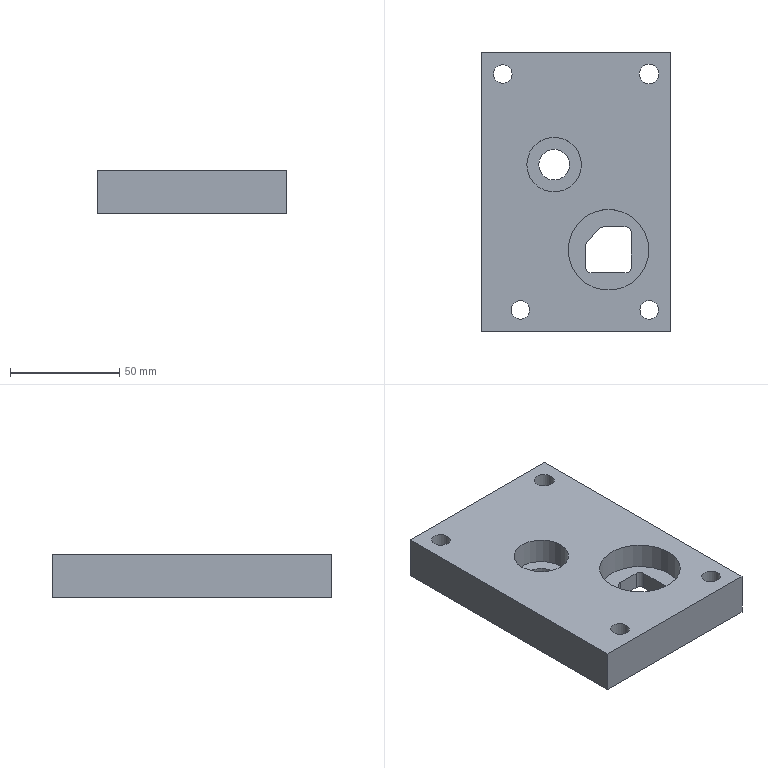Part | NX | features solid 2 | 1 solid | 33 faces | box 87 x 128 x 20 mm | volume 190901 mm3 | plane 17 | cylinder 16 | commonest cylinder face diameters 5 x5 14 x4 8.5 x3 9 x1 14.1 x1 25 x1
STEP:
#1=CARTESIAN_POINT('',(137.75,-206.5,20.));
#2=VERTEX_POINT('',#1);
#3=CARTESIAN_POINT('',(133.5,-206.5,20.));
#4=DIRECTION('',(0.,0.,1.));
#5=DIRECTION('',(1.,0.,0.));
#6=AXIS2_PLACEMENT_3D('',#3,#4,#5);
#7=CIRCLE('',#6,4.25);
#8=EDGE_CURVE('',#2,#2,#7,.F.);
#9=ORIENTED_EDGE('',*,*,#8,.T.);
#10=EDGE_LOOP('',(#9));
#11=FACE_BOUND('',#10,.T.);
#12=CARTESIAN_POINT('',(121.25,-98.5,20.));
#13=VERTEX_POINT('',#12);
#14=CARTESIAN_POINT('',(125.5,-98.5,20.));
#15=DIRECTION('',(0.,0.,1.));
#16=DIRECTION('',(-1.,0.,0.));
#17=AXIS2_PLACEMENT_3D('',#14,#15,#16);
#18=CIRCLE('',#17,4.25);
#19=EDGE_CURVE('',#13,#13,#18,.T.);
#20=ORIENTED_EDGE('',*,*,#19,.F.);
#21=EDGE_LOOP('',(#20));
#22=FACE_BOUND('',#21,.T.);
#23=CARTESIAN_POINT('',(196.75,-206.5,20.));
#24=VERTEX_POINT('',#23);
#25=CARTESIAN_POINT('',(192.5,-206.5,20.));
#26=DIRECTION('',(0.,0.,1.));
#27=DIRECTION('',(1.,0.,0.));
#28=AXIS2_PLACEMENT_3D('',#25,#26,#27);
#29=CIRCLE('',#28,4.25);
#30=EDGE_CURVE('',#24,#24,#29,.T.);
#31=ORIENTED_EDGE('',*,*,#30,.F.);
#32=EDGE_LOOP('',(#31));
#33=FACE_BOUND('',#32,.T.);
#34=CARTESIAN_POINT('',(197.,-98.5,20.));
#35=VERTEX_POINT('',#34);
#36=CARTESIAN_POINT('',(192.5,-98.5,20.));
#37=DIRECTION('',(0.,0.,-1.));
#38=DIRECTION('',(1.,0.,0.));
#39=AXIS2_PLACEMENT_3D('',#36,#37,#38);
#40=CIRCLE('',#39,4.5);
#41=EDGE_CURVE('',#35,#35,#40,.F.);
#42=ORIENTED_EDGE('',*,*,#41,.F.);
#43=EDGE_LOOP('',(#42));
#44=FACE_BOUND('',#43,.T.);
#45=CARTESIAN_POINT('',(202.5,-216.5,20.));
#46=VERTEX_POINT('',#45);
#47=CARTESIAN_POINT('',(115.5,-216.5,20.));
#48=VERTEX_POINT('',#47);
#49=CARTESIAN_POINT('',(149.,-216.5,20.));
#50=DIRECTION('',(1.,0.,0.));
#51=VECTOR('',#50,1000.);
#52=LINE('',#49,#51);
#53=EDGE_CURVE('',#46,#48,#52,.F.);
#54=ORIENTED_EDGE('',*,*,#53,.F.);
#55=CARTESIAN_POINT('',(202.5,-88.5,20.));
#56=VERTEX_POINT('',#55);
#57=CARTESIAN_POINT('',(202.5,-140.,20.));
#58=DIRECTION('',(0.,-1.,0.));
#59=VECTOR('',#58,1000.);
#60=LINE('',#57,#59);
#61=EDGE_CURVE('',#56,#46,#60,.T.);
#62=ORIENTED_EDGE('',*,*,#61,.F.);
#63=CARTESIAN_POINT('',(115.5,-88.5,20.));
#64=VERTEX_POINT('',#63);
#65=CARTESIAN_POINT('',(149.,-88.5,20.));
#66=DIRECTION('',(1.,0.,0.));
#67=VECTOR('',#66,1000.);
#68=LINE('',#65,#67);
#69=EDGE_CURVE('',#64,#56,#68,.T.);
#70=ORIENTED_EDGE('',*,*,#69,.F.);
#71=CARTESIAN_POINT('',(115.5,-140.,20.));
#72=DIRECTION('',(0.,1.,0.));
#73=VECTOR('',#72,1000.);
#74=LINE('',#71,#73);
#75=EDGE_CURVE('',#48,#64,#74,.T.);
#76=ORIENTED_EDGE('',*,*,#75,.F.);
#77=EDGE_LOOP('',(#54,#62,#70,#76));
#78=FACE_BOUND('',#77,.T.);
#79=CARTESIAN_POINT('',(161.5,-140.,20.));
#80=VERTEX_POINT('',#79);
#81=CARTESIAN_POINT('',(149.,-140.,20.));
#82=DIRECTION('',(0.,0.,1.));
#83=DIRECTION('',(1.,0.,0.));
#84=AXIS2_PLACEMENT_3D('',#81,#82,#83);
#85=CIRCLE('',#84,12.5);
#86=EDGE_CURVE('',#80,#80,#85,.T.);
#87=ORIENTED_EDGE('',*,*,#86,.F.);
#88=EDGE_LOOP('',(#87));
#89=FACE_BOUND('',#88,.T.);
#90=CARTESIAN_POINT('',(192.401,-179.,20.));
#91=VERTEX_POINT('',#90);
#92=CARTESIAN_POINT('',(173.901,-179.,20.));
#93=DIRECTION('',(0.,0.,1.));
#94=DIRECTION('',(1.,0.,0.));
#95=AXIS2_PLACEMENT_3D('',#92,#93,#94);
#96=CIRCLE('',#95,18.5);
#97=EDGE_CURVE('',#91,#91,#96,.T.);
#98=ORIENTED_EDGE('',*,*,#97,.F.);
#99=EDGE_LOOP('',(#98));
#100=FACE_BOUND('',#99,.T.);
#101=CARTESIAN_POINT('',(251.29,-25.984,20.));
#102=DIRECTION('',(0.,0.,1.));
#103=DIRECTION('',(1.,0.,0.));
#104=AXIS2_PLACEMENT_3D('',#101,#102,#103);
#105=PLANE('',#104);
#106=ADVANCED_FACE('',(#11,#22,#33,#44,#78,#89,#100),#105,.T.);
#107=CARTESIAN_POINT('',(185.5,-98.5,0.00000121));
#108=VERTEX_POINT('',#107);
#109=CARTESIAN_POINT('',(192.5,-98.5,0.00000121));
#110=DIRECTION('',(0.,0.,1.));
#111=DIRECTION('',(-1.,0.,0.));
#112=AXIS2_PLACEMENT_3D('',#109,#110,#111);
#113=CIRCLE('',#112,7.);
#114=EDGE_CURVE('',#108,#108,#113,.F.);
#115=ORIENTED_EDGE('',*,*,#114,.F.);
#116=EDGE_LOOP('',(#115));
#117=FACE_BOUND('',#116,.T.);
#118=CARTESIAN_POINT('',(141.95,-140.,0.00000121));
#119=VERTEX_POINT('',#118);
#120=CARTESIAN_POINT('',(149.,-140.,0.00000121));
#121=DIRECTION('',(0.,0.,1.));
#122=DIRECTION('',(-1.,0.,0.));
#123=AXIS2_PLACEMENT_3D('',#120,#121,#122);
#124=CIRCLE('',#123,7.05);
#125=EDGE_CURVE('',#119,#119,#124,.F.);
#126=ORIENTED_EDGE('',*,*,#125,.F.);
#127=EDGE_LOOP('',(#126));
#128=FACE_BOUND('',#127,.T.);
#129=CARTESIAN_POINT('',(185.5,-206.5,0.00000121));
#130=VERTEX_POINT('',#129);
#131=CARTESIAN_POINT('',(192.5,-206.5,0.00000121));
#132=DIRECTION('',(0.,0.,-1.));
#133=DIRECTION('',(-1.,0.,0.));
#134=AXIS2_PLACEMENT_3D('',#131,#132,#133);
#135=CIRCLE('',#134,7.);
#136=EDGE_CURVE('',#130,#130,#135,.T.);
#137=ORIENTED_EDGE('',*,*,#136,.F.);
#138=EDGE_LOOP('',(#137));
#139=FACE_BOUND('',#138,.T.);
#140=CARTESIAN_POINT('',(202.5,-88.5,0.00000121));
#141=VERTEX_POINT('',#140);
#142=CARTESIAN_POINT('',(202.5,-216.5,0.00000121));
#143=VERTEX_POINT('',#142);
#144=CARTESIAN_POINT('',(202.5,-140.,0.00000121));
#145=DIRECTION('',(0.,1.,0.));
#146=VECTOR('',#145,1000.);
#147=LINE('',#144,#146);
#148=EDGE_CURVE('',#141,#143,#147,.F.);
#149=ORIENTED_EDGE('',*,*,#148,.T.);
#150=CARTESIAN_POINT('',(115.5,-216.5,0.00000121));
#151=VERTEX_POINT('',#150);
#152=CARTESIAN_POINT('',(149.,-216.5,0.00000121));
#153=DIRECTION('',(-1.,0.,0.));
#154=VECTOR('',#153,1000.);
#155=LINE('',#152,#154);
#156=EDGE_CURVE('',#143,#151,#155,.T.);
#157=ORIENTED_EDGE('',*,*,#156,.T.);
#158=CARTESIAN_POINT('',(115.5,-88.5,0.00000121));
#159=VERTEX_POINT('',#158);
#160=CARTESIAN_POINT('',(115.5,-140.,0.00000121));
#161=DIRECTION('',(0.,-1.,0.));
#162=VECTOR('',#161,1000.);
#163=LINE('',#160,#162);
#164=EDGE_CURVE('',#151,#159,#163,.F.);
#165=ORIENTED_EDGE('',*,*,#164,.T.);
#166=CARTESIAN_POINT('',(149.,-88.5,0.00000121));
#167=DIRECTION('',(-1.,0.,0.));
#168=VECTOR('',#167,1000.);
#169=LINE('',#166,#168);
#170=EDGE_CURVE('',#159,#141,#169,.F.);
#171=ORIENTED_EDGE('',*,*,#170,.T.);
#172=EDGE_LOOP('',(#149,#157,#165,#171));
#173=FACE_BOUND('',#172,.T.);
#174=CARTESIAN_POINT('',(132.5,-98.5,0.00000121));
#175=VERTEX_POINT('',#174);
#176=CARTESIAN_POINT('',(125.5,-98.5,0.00000121));
#177=DIRECTION('',(0.,0.,-1.));
#178=DIRECTION('',(1.,0.,0.));
#179=AXIS2_PLACEMENT_3D('',#176,#177,#178);
#180=CIRCLE('',#179,7.);
#181=EDGE_CURVE('',#175,#175,#180,.T.);
#182=ORIENTED_EDGE('',*,*,#181,.F.);
#183=EDGE_LOOP('',(#182));
#184=FACE_BOUND('',#183,.T.);
#185=CARTESIAN_POINT('',(126.5,-206.5,0.00000121));
#186=VERTEX_POINT('',#185);
#187=CARTESIAN_POINT('',(133.5,-206.5,0.00000121));
#188=DIRECTION('',(0.,0.,-1.));
#189=DIRECTION('',(-1.,0.,0.));
#190=AXIS2_PLACEMENT_3D('',#187,#188,#189);
#191=CIRCLE('',#190,7.);
#192=EDGE_CURVE('',#186,#186,#191,.T.);
#193=ORIENTED_EDGE('',*,*,#192,.F.);
#194=EDGE_LOOP('',(#193));
#195=FACE_BOUND('',#194,.T.);
#196=CARTESIAN_POINT('',(184.401,-171.,0.00000121));
#197=VERTEX_POINT('',#196);
#198=CARTESIAN_POINT('',(181.901,-168.5,0.00000121));
#199=VERTEX_POINT('',#198);
#200=CARTESIAN_POINT('',(181.901,-171.,0.00000121));
#201=DIRECTION('',(0.,0.,-1.));
#202=DIRECTION('',(-1.,0.,0.));
#203=AXIS2_PLACEMENT_3D('',#200,#201,#202);
#204=CIRCLE('',#203,2.5);
#205=EDGE_CURVE('',#197,#199,#204,.F.);
#206=ORIENTED_EDGE('',*,*,#205,.T.);
#207=CARTESIAN_POINT('',(171.729,-168.5,0.00000121));
#208=VERTEX_POINT('',#207);
#209=CARTESIAN_POINT('',(149.,-168.5,0.00000121));
#210=DIRECTION('',(-1.,0.,0.));
#211=VECTOR('',#210,1000.);
#212=LINE('',#209,#211);
#213=EDGE_CURVE('',#199,#208,#212,.T.);
#214=ORIENTED_EDGE('',*,*,#213,.T.);
#215=CARTESIAN_POINT('',(169.961,-169.232,0.00000121));
#216=VERTEX_POINT('',#215);
#217=CARTESIAN_POINT('',(171.729,-171.,0.00000121));
#218=DIRECTION('',(0.,0.,-1.));
#219=DIRECTION('',(-1.,0.,0.));
#220=AXIS2_PLACEMENT_3D('',#217,#218,#219);
#221=CIRCLE('',#220,2.5);
#222=EDGE_CURVE('',#208,#216,#221,.F.);
#223=ORIENTED_EDGE('',*,*,#222,.T.);
#224=CARTESIAN_POINT('',(164.133,-175.061,0.00000121));
#225=VERTEX_POINT('',#224);
#226=CARTESIAN_POINT('',(174.097,-165.097,0.00000121));
#227=DIRECTION('',(-0.7071,-0.7071,0.));
#228=VECTOR('',#227,1000.);
#229=LINE('',#226,#228);
#230=EDGE_CURVE('',#216,#225,#229,.T.);
#231=ORIENTED_EDGE('',*,*,#230,.T.);
#232=CARTESIAN_POINT('',(163.401,-176.828,0.00000121));
#233=VERTEX_POINT('',#232);
#234=CARTESIAN_POINT('',(165.901,-176.828,0.00000121));
#235=DIRECTION('',(0.,0.,-1.));
#236=DIRECTION('',(-1.,0.,0.));
#237=AXIS2_PLACEMENT_3D('',#234,#235,#236);
#238=CIRCLE('',#237,2.5);
#239=EDGE_CURVE('',#225,#233,#238,.F.);
#240=ORIENTED_EDGE('',*,*,#239,.T.);
#241=CARTESIAN_POINT('',(163.401,-187.,0.00000121));
#242=VERTEX_POINT('',#241);
#243=CARTESIAN_POINT('',(163.401,-140.,0.00000121));
#244=DIRECTION('',(0.,-1.,0.));
#245=VECTOR('',#244,1000.);
#246=LINE('',#243,#245);
#247=EDGE_CURVE('',#233,#242,#246,.T.);
#248=ORIENTED_EDGE('',*,*,#247,.T.);
#249=CARTESIAN_POINT('',(165.901,-189.5,0.00000121));
#250=VERTEX_POINT('',#249);
#251=CARTESIAN_POINT('',(165.901,-187.,0.00000121));
#252=DIRECTION('',(0.,0.,-1.));
#253=DIRECTION('',(-1.,0.,0.));
#254=AXIS2_PLACEMENT_3D('',#251,#252,#253);
#255=CIRCLE('',#254,2.5);
#256=EDGE_CURVE('',#242,#250,#255,.F.);
#257=ORIENTED_EDGE('',*,*,#256,.T.);
#258=CARTESIAN_POINT('',(181.901,-189.5,0.00000121));
#259=VERTEX_POINT('',#258);
#260=CARTESIAN_POINT('',(149.,-189.5,0.00000121));
#261=DIRECTION('',(1.,0.,0.));
#262=VECTOR('',#261,1000.);
#263=LINE('',#260,#262);
#264=EDGE_CURVE('',#250,#259,#263,.T.);
#265=ORIENTED_EDGE('',*,*,#264,.T.);
#266=CARTESIAN_POINT('',(184.401,-187.,0.00000121));
#267=VERTEX_POINT('',#266);
#268=CARTESIAN_POINT('',(181.901,-187.,0.00000121));
#269=DIRECTION('',(0.,0.,-1.));
#270=DIRECTION('',(-1.,0.,0.));
#271=AXIS2_PLACEMENT_3D('',#268,#269,#270);
#272=CIRCLE('',#271,2.5);
#273=EDGE_CURVE('',#259,#267,#272,.F.);
#274=ORIENTED_EDGE('',*,*,#273,.T.);
#275=CARTESIAN_POINT('',(184.401,-140.,0.00000121));
#276=DIRECTION('',(0.,1.,0.));
#277=VECTOR('',#276,1000.);
#278=LINE('',#275,#277);
#279=EDGE_CURVE('',#267,#197,#278,.T.);
#280=ORIENTED_EDGE('',*,*,#279,.T.);
#281=EDGE_LOOP('',(#206,#214,#223,#231,#240,#248,#257,#265,#274,#280));
#282=FACE_BOUND('',#281,.T.);
#283=CARTESIAN_POINT('',(149.,-140.,0.00000121));
#284=DIRECTION('',(0.,0.,-1.));
#285=DIRECTION('',(-1.,0.,0.));
#286=AXIS2_PLACEMENT_3D('',#283,#284,#285);
#287=PLANE('',#286);
#288=ADVANCED_FACE('',(#117,#128,#139,#173,#184,#195,#282),#287,.T.);
#289=CARTESIAN_POINT('',(129.25,-206.5,10.));
#290=VERTEX_POINT('',#289);
#291=CARTESIAN_POINT('',(133.5,-206.5,10.));
#292=DIRECTION('',(0.,0.,-1.));
#293=DIRECTION('',(-1.,0.,0.));
#294=AXIS2_PLACEMENT_3D('',#291,#292,#293);
#295=CIRCLE('',#294,4.25);
#296=EDGE_CURVE('',#290,#290,#295,.F.);
#297=ORIENTED_EDGE('',*,*,#296,.T.);
#298=EDGE_LOOP('',(#297));
#299=FACE_BOUND('',#298,.T.);
#300=CARTESIAN_POINT('',(126.5,-206.5,10.));
#301=VERTEX_POINT('',#300);
#302=CARTESIAN_POINT('',(133.5,-206.5,10.));
#303=DIRECTION('',(0.,0.,-1.));
#304=DIRECTION('',(-1.,0.,0.));
#305=AXIS2_PLACEMENT_3D('',#302,#303,#304);
#306=CIRCLE('',#305,7.);
#307=EDGE_CURVE('',#301,#301,#306,.F.);
#308=ORIENTED_EDGE('',*,*,#307,.F.);
#309=EDGE_LOOP('',(#308));
#310=FACE_BOUND('',#309,.T.);
#311=CARTESIAN_POINT('',(19.595,-220.431,10.));
#312=DIRECTION('',(0.,0.,1.));
#313=DIRECTION('',(-1.,0.,0.));
#314=AXIS2_PLACEMENT_3D('',#311,#312,#313);
#315=PLANE('',#314);
#316=ADVANCED_FACE('',(#299,#310),#315,.F.);
#317=ORIENTED_EDGE('',*,*,#8,.F.);
#318=EDGE_LOOP('',(#317));
#319=FACE_BOUND('',#318,.T.);
#320=ORIENTED_EDGE('',*,*,#296,.F.);
#321=EDGE_LOOP('',(#320));
#322=FACE_BOUND('',#321,.T.);
#323=CARTESIAN_POINT('',(133.5,-206.5,35.));
#324=DIRECTION('',(0.,0.,1.));
#325=DIRECTION('',(1.,0.,0.));
#326=AXIS2_PLACEMENT_3D('',#323,#324,#325);
#327=CYLINDRICAL_SURFACE('',#326,4.25);
#328=ADVANCED_FACE('',(#319,#322),#327,.F.);
#329=ORIENTED_EDGE('',*,*,#307,.T.);
#330=EDGE_LOOP('',(#329));
#331=FACE_BOUND('',#330,.T.);
#332=ORIENTED_EDGE('',*,*,#192,.T.);
#333=EDGE_LOOP('',(#332));
#334=FACE_BOUND('',#333,.T.);
#335=CARTESIAN_POINT('',(133.5,-206.5,0.00000121));
#336=DIRECTION('',(0.,0.,1.));
#337=DIRECTION('',(1.,0.,0.));
#338=AXIS2_PLACEMENT_3D('',#335,#336,#337);
#339=CYLINDRICAL_SURFACE('',#338,7.);
#340=ADVANCED_FACE('',(#331,#334),#339,.F.);
#341=CARTESIAN_POINT('',(197.,-98.5,10.));
#342=VERTEX_POINT('',#341);
#343=CARTESIAN_POINT('',(192.5,-98.5,10.));
#344=DIRECTION('',(0.,0.,-1.));
#345=DIRECTION('',(1.,0.,0.));
#346=AXIS2_PLACEMENT_3D('',#343,#344,#345);
#347=CIRCLE('',#346,4.5);
#348=EDGE_CURVE('',#342,#342,#347,.F.);
#349=ORIENTED_EDGE('',*,*,#348,.T.);
#350=EDGE_LOOP('',(#349));
#351=FACE_BOUND('',#350,.T.);
#352=CARTESIAN_POINT('',(199.5,-98.5,10.));
#353=VERTEX_POINT('',#352);
#354=CARTESIAN_POINT('',(192.5,-98.5,10.));
#355=DIRECTION('',(0.,0.,-1.));
#356=DIRECTION('',(1.,0.,0.));
#357=AXIS2_PLACEMENT_3D('',#354,#355,#356);
#358=CIRCLE('',#357,7.);
#359=EDGE_CURVE('',#353,#353,#358,.F.);
#360=ORIENTED_EDGE('',*,*,#359,.F.);
#361=EDGE_LOOP('',(#360));
#362=FACE_BOUND('',#361,.T.);
#363=CARTESIAN_POINT('',(306.405,-84.569,10.));
#364=DIRECTION('',(0.,0.,1.));
#365=DIRECTION('',(1.,0.,0.));
#366=AXIS2_PLACEMENT_3D('',#363,#364,#365);
#367=PLANE('',#366);
#368=ADVANCED_FACE('',(#351,#362),#367,.F.);
#369=CARTESIAN_POINT('',(161.5,-140.,8.));
#370=VERTEX_POINT('',#369);
#371=CARTESIAN_POINT('',(149.,-140.,8.));
#372=DIRECTION('',(0.,0.,1.));
#373=DIRECTION('',(1.,0.,0.));
#374=AXIS2_PLACEMENT_3D('',#371,#372,#373);
#375=CIRCLE('',#374,12.5);
#376=EDGE_CURVE('',#370,#370,#375,.T.);
#377=ORIENTED_EDGE('',*,*,#376,.T.);
#378=EDGE_LOOP('',(#377));
#379=FACE_BOUND('',#378,.T.);
#380=CARTESIAN_POINT('',(156.05,-140.,8.));
#381=VERTEX_POINT('',#380);
#382=CARTESIAN_POINT('',(149.,-140.,8.));
#383=DIRECTION('',(0.,0.,1.));
#384=DIRECTION('',(1.,0.,0.));
#385=AXIS2_PLACEMENT_3D('',#382,#383,#384);
#386=CIRCLE('',#385,7.05);
#387=EDGE_CURVE('',#381,#381,#386,.F.);
#388=ORIENTED_EDGE('',*,*,#387,.T.);
#389=EDGE_LOOP('',(#388));
#390=FACE_BOUND('',#389,.T.);
#391=CARTESIAN_POINT('',(151.5,140.,8.));
#392=DIRECTION('',(0.,0.,1.));
#393=DIRECTION('',(1.,0.,0.));
#394=AXIS2_PLACEMENT_3D('',#391,#392,#393);
#395=PLANE('',#394);
#396=ADVANCED_FACE('',(#379,#390),#395,.T.);
#397=CARTESIAN_POINT('',(196.75,-206.5,10.));
#398=VERTEX_POINT('',#397);
#399=CARTESIAN_POINT('',(192.5,-206.5,10.));
#400=DIRECTION('',(0.,0.,1.));
#401=DIRECTION('',(1.,0.,0.));
#402=AXIS2_PLACEMENT_3D('',#399,#400,#401);
#403=CIRCLE('',#402,4.25);
#404=EDGE_CURVE('',#398,#398,#403,.T.);
#405=ORIENTED_EDGE('',*,*,#404,.T.);
#406=EDGE_LOOP('',(#405));
#407=FACE_BOUND('',#406,.T.);
#408=CARTESIAN_POINT('',(199.5,-206.5,10.));
#409=VERTEX_POINT('',#408);
#410=CARTESIAN_POINT('',(192.5,-206.5,10.));
#411=DIRECTION('',(0.,0.,1.));
#412=DIRECTION('',(1.,0.,0.));
#413=AXIS2_PLACEMENT_3D('',#410,#411,#412);
#414=CIRCLE('',#413,7.);
#415=EDGE_CURVE('',#409,#409,#414,.T.);
#416=ORIENTED_EDGE('',*,*,#415,.F.);
#417=EDGE_LOOP('',(#416));
#418=FACE_BOUND('',#417,.T.);
#419=CARTESIAN_POINT('',(306.405,-220.431,10.));
#420=DIRECTION('',(0.,0.,1.));
#421=DIRECTION('',(1.,0.,0.));
#422=AXIS2_PLACEMENT_3D('',#419,#420,#421);
#423=PLANE('',#422);
#424=ADVANCED_FACE('',(#407,#418),#423,.F.);
#425=CARTESIAN_POINT('',(121.25,-98.5,10.));
#426=VERTEX_POINT('',#425);
#427=CARTESIAN_POINT('',(125.5,-98.5,10.));
#428=DIRECTION('',(0.,0.,1.));
#429=DIRECTION('',(-1.,0.,0.));
#430=AXIS2_PLACEMENT_3D('',#427,#428,#429);
#431=CIRCLE('',#430,4.25);
#432=EDGE_CURVE('',#426,#426,#431,.T.);
#433=ORIENTED_EDGE('',*,*,#432,.T.);
#434=EDGE_LOOP('',(#433));
#435=FACE_BOUND('',#434,.T.);
#436=CARTESIAN_POINT('',(118.5,-98.5,10.));
#437=VERTEX_POINT('',#436);
#438=CARTESIAN_POINT('',(125.5,-98.5,10.));
#439=DIRECTION('',(0.,0.,1.));
#440=DIRECTION('',(-1.,0.,0.));
#441=AXIS2_PLACEMENT_3D('',#438,#439,#440);
#442=CIRCLE('',#441,7.);
#443=EDGE_CURVE('',#437,#437,#442,.T.);
#444=ORIENTED_EDGE('',*,*,#443,.F.);
#445=EDGE_LOOP('',(#444));
#446=FACE_BOUND('',#445,.T.);
#447=CARTESIAN_POINT('',(11.595,-84.569,10.));
#448=DIRECTION('',(0.,0.,1.));
#449=DIRECTION('',(-1.,0.,0.));
#450=AXIS2_PLACEMENT_3D('',#447,#448,#449);
#451=PLANE('',#450);
#452=ADVANCED_FACE('',(#435,#446),#451,.F.);
#453=ORIENTED_EDGE('',*,*,#376,.F.);
#454=EDGE_LOOP('',(#453));
#455=FACE_BOUND('',#454,.T.);
#456=ORIENTED_EDGE('',*,*,#86,.T.);
#457=EDGE_LOOP('',(#456));
#458=FACE_BOUND('',#457,.T.);
#459=CARTESIAN_POINT('',(149.,-140.,2.5));
#460=DIRECTION('',(0.,0.,-1.));
#461=DIRECTION('',(-1.,0.,0.));
#462=AXIS2_PLACEMENT_3D('',#459,#460,#461);
#463=CYLINDRICAL_SURFACE('',#462,12.5);
#464=ADVANCED_FACE('',(#455,#458),#463,.F.);
#465=ORIENTED_EDGE('',*,*,#359,.T.);
#466=EDGE_LOOP('',(#465));
#467=FACE_BOUND('',#466,.T.);
#468=ORIENTED_EDGE('',*,*,#114,.T.);
#469=EDGE_LOOP('',(#468));
#470=FACE_BOUND('',#469,.T.);
#471=CARTESIAN_POINT('',(192.5,-98.5,0.00000121));
#472=DIRECTION('',(0.,0.,1.));
#473=DIRECTION('',(-1.,0.,0.));
#474=AXIS2_PLACEMENT_3D('',#471,#472,#473);
#475=CYLINDRICAL_SURFACE('',#474,7.);
#476=ADVANCED_FACE('',(#467,#470),#475,.F.);
#477=ORIENTED_EDGE('',*,*,#125,.T.);
#478=EDGE_LOOP('',(#477));
#479=FACE_BOUND('',#478,.T.);
#480=ORIENTED_EDGE('',*,*,#387,.F.);
#481=EDGE_LOOP('',(#480));
#482=FACE_BOUND('',#481,.T.);
#483=CARTESIAN_POINT('',(149.,-140.,2.5));
#484=DIRECTION('',(0.,0.,-1.));
#485=DIRECTION('',(-1.,0.,0.));
#486=AXIS2_PLACEMENT_3D('',#483,#484,#485);
#487=CYLINDRICAL_SURFACE('',#486,7.05);
#488=ADVANCED_FACE('',(#479,#482),#487,.F.);
#489=ORIENTED_EDGE('',*,*,#415,.T.);
#490=EDGE_LOOP('',(#489));
#491=FACE_BOUND('',#490,.T.);
#492=ORIENTED_EDGE('',*,*,#136,.T.);
#493=EDGE_LOOP('',(#492));
#494=FACE_BOUND('',#493,.T.);
#495=CARTESIAN_POINT('',(192.5,-206.5,0.00000121));
#496=DIRECTION('',(0.,0.,1.));
#497=DIRECTION('',(-1.,0.,0.));
#498=AXIS2_PLACEMENT_3D('',#495,#496,#497);
#499=CYLINDRICAL_SURFACE('',#498,7.);
#500=ADVANCED_FACE('',(#491,#494),#499,.F.);
#501=CARTESIAN_POINT('',(202.5,-88.5,35.));
#502=DIRECTION('',(0.,0.,-1.));
#503=VECTOR('',#502,1000.);
#504=LINE('',#501,#503);
#505=EDGE_CURVE('',#56,#141,#504,.T.);
#506=ORIENTED_EDGE('',*,*,#505,.T.);
#507=ORIENTED_EDGE('',*,*,#170,.F.);
#508=CARTESIAN_POINT('',(115.5,-88.5,35.));
#509=DIRECTION('',(0.,0.,-1.));
#510=VECTOR('',#509,1000.);
#511=LINE('',#508,#510);
#512=EDGE_CURVE('',#64,#159,#511,.T.);
#513=ORIENTED_EDGE('',*,*,#512,.F.);
#514=ORIENTED_EDGE('',*,*,#69,.T.);
#515=EDGE_LOOP('',(#506,#507,#513,#514));
#516=FACE_BOUND('',#515,.T.);
#517=CARTESIAN_POINT('',(149.,-88.5,35.));
#518=DIRECTION('',(0.,-1.,0.));
#519=DIRECTION('',(1.,0.,0.));
#520=AXIS2_PLACEMENT_3D('',#517,#518,#519);
#521=PLANE('',#520);
#522=ADVANCED_FACE('',(#516),#521,.F.);
#523=ORIENTED_EDGE('',*,*,#512,.T.);
#524=ORIENTED_EDGE('',*,*,#164,.F.);
#525=CARTESIAN_POINT('',(115.5,-216.5,35.));
#526=DIRECTION('',(0.,0.,-1.));
#527=VECTOR('',#526,1000.);
#528=LINE('',#525,#527);
#529=EDGE_CURVE('',#151,#48,#528,.F.);
#530=ORIENTED_EDGE('',*,*,#529,.T.);
#531=ORIENTED_EDGE('',*,*,#75,.T.);
#532=EDGE_LOOP('',(#523,#524,#530,#531));
#533=FACE_BOUND('',#532,.T.);
#534=CARTESIAN_POINT('',(115.5,-140.,35.));
#535=DIRECTION('',(1.,0.,0.));
#536=DIRECTION('',(0.,1.,0.));
#537=AXIS2_PLACEMENT_3D('',#534,#535,#536);
#538=PLANE('',#537);
#539=ADVANCED_FACE('',(#533),#538,.F.);
#540=ORIENTED_EDGE('',*,*,#529,.F.);
#541=ORIENTED_EDGE('',*,*,#156,.F.);
#542=CARTESIAN_POINT('',(202.5,-216.5,35.));
#543=DIRECTION('',(0.,0.,-1.));
#544=VECTOR('',#543,1000.);
#545=LINE('',#542,#544);
#546=EDGE_CURVE('',#46,#143,#545,.T.);
#547=ORIENTED_EDGE('',*,*,#546,.F.);
#548=ORIENTED_EDGE('',*,*,#53,.T.);
#549=EDGE_LOOP('',(#540,#541,#547,#548));
#550=FACE_BOUND('',#549,.T.);
#551=CARTESIAN_POINT('',(149.,-216.5,35.));
#552=DIRECTION('',(0.,1.,0.));
#553=DIRECTION('',(-1.,0.,0.));
#554=AXIS2_PLACEMENT_3D('',#551,#552,#553);
#555=PLANE('',#554);
#556=ADVANCED_FACE('',(#550),#555,.F.);
#557=ORIENTED_EDGE('',*,*,#546,.T.);
#558=ORIENTED_EDGE('',*,*,#148,.F.);
#559=ORIENTED_EDGE('',*,*,#505,.F.);
#560=ORIENTED_EDGE('',*,*,#61,.T.);
#561=EDGE_LOOP('',(#557,#558,#559,#560));
#562=FACE_BOUND('',#561,.T.);
#563=CARTESIAN_POINT('',(202.5,-140.,35.));
#564=DIRECTION('',(-1.,0.,0.));
#565=DIRECTION('',(0.,-1.,0.));
#566=AXIS2_PLACEMENT_3D('',#563,#564,#565);
#567=PLANE('',#566);
#568=ADVANCED_FACE('',(#562),#567,.F.);
#569=ORIENTED_EDGE('',*,*,#443,.T.);
#570=EDGE_LOOP('',(#569));
#571=FACE_BOUND('',#570,.T.);
#572=ORIENTED_EDGE('',*,*,#181,.T.);
#573=EDGE_LOOP('',(#572));
#574=FACE_BOUND('',#573,.T.);
#575=CARTESIAN_POINT('',(125.5,-98.5,0.00000121));
#576=DIRECTION('',(0.,0.,1.));
#577=DIRECTION('',(1.,0.,0.));
#578=AXIS2_PLACEMENT_3D('',#575,#576,#577);
#579=CYLINDRICAL_SURFACE('',#578,7.);
#580=ADVANCED_FACE('',(#571,#574),#579,.F.);
#581=ORIENTED_EDGE('',*,*,#41,.T.);
#582=EDGE_LOOP('',(#581));
#583=FACE_BOUND('',#582,.T.);
#584=ORIENTED_EDGE('',*,*,#348,.F.);
#585=EDGE_LOOP('',(#584));
#586=FACE_BOUND('',#585,.T.);
#587=CARTESIAN_POINT('',(192.5,-98.5,35.));
#588=DIRECTION('',(0.,0.,1.));
#589=DIRECTION('',(-1.,0.,0.));
#590=AXIS2_PLACEMENT_3D('',#587,#588,#589);
#591=CYLINDRICAL_SURFACE('',#590,4.5);
#592=ADVANCED_FACE('',(#583,#586),#591,.F.);
#593=ORIENTED_EDGE('',*,*,#30,.T.);
#594=EDGE_LOOP('',(#593));
#595=FACE_BOUND('',#594,.T.);
#596=ORIENTED_EDGE('',*,*,#404,.F.);
#597=EDGE_LOOP('',(#596));
#598=FACE_BOUND('',#597,.T.);
#599=CARTESIAN_POINT('',(192.5,-206.5,35.));
#600=DIRECTION('',(0.,0.,1.));
#601=DIRECTION('',(-1.,0.,0.));
#602=AXIS2_PLACEMENT_3D('',#599,#600,#601);
#603=CYLINDRICAL_SURFACE('',#602,4.25);
#604=ADVANCED_FACE('',(#595,#598),#603,.F.);
#605=ORIENTED_EDGE('',*,*,#19,.T.);
#606=EDGE_LOOP('',(#605));
#607=FACE_BOUND('',#606,.T.);
#608=ORIENTED_EDGE('',*,*,#432,.F.);
#609=EDGE_LOOP('',(#608));
#610=FACE_BOUND('',#609,.T.);
#611=CARTESIAN_POINT('',(125.5,-98.5,35.));
#612=DIRECTION('',(0.,0.,1.));
#613=DIRECTION('',(1.,0.,0.));
#614=AXIS2_PLACEMENT_3D('',#611,#612,#613);
#615=CYLINDRICAL_SURFACE('',#614,4.25);
#616=ADVANCED_FACE('',(#607,#610),#615,.F.);
#617=CARTESIAN_POINT('',(171.729,-168.5,8.));
#618=VERTEX_POINT('',#617);
#619=CARTESIAN_POINT('',(181.901,-168.5,8.));
#620=VERTEX_POINT('',#619);
#621=CARTESIAN_POINT('',(171.729,-168.5,8.));
#622=DIRECTION('',(1.,0.,0.));
#623=VECTOR('',#622,1000.);
#624=LINE('',#621,#623);
#625=EDGE_CURVE('',#618,#620,#624,.T.);
#626=ORIENTED_EDGE('',*,*,#625,.F.);
#627=CARTESIAN_POINT('',(171.729,-168.5,-64.));
#628=DIRECTION('',(0.,0.,1.));
#629=VECTOR('',#628,1000.);
#630=LINE('',#627,#629);
#631=EDGE_CURVE('',#618,#208,#630,.F.);
#632=ORIENTED_EDGE('',*,*,#631,.T.);
#633=ORIENTED_EDGE('',*,*,#213,.F.);
#634=CARTESIAN_POINT('',(181.901,-168.5,-64.));
#635=DIRECTION('',(0.,0.,1.));
#636=VECTOR('',#635,1000.);
#637=LINE('',#634,#636);
#638=EDGE_CURVE('',#620,#199,#637,.F.);
#639=ORIENTED_EDGE('',*,*,#638,.F.);
#640=EDGE_LOOP('',(#626,#632,#633,#639));
#641=FACE_BOUND('',#640,.T.);
#642=CARTESIAN_POINT('',(171.729,-168.5,-64.));
#643=DIRECTION('',(0.,-1.,0.));
#644=DIRECTION('',(1.,0.,0.));
#645=AXIS2_PLACEMENT_3D('',#642,#643,#644);
#646=PLANE('',#645);
#647=ADVANCED_FACE('',(#641),#646,.T.);
#648=CARTESIAN_POINT('',(184.401,-171.,8.));
#649=VERTEX_POINT('',#648);
#650=CARTESIAN_POINT('',(181.901,-171.,8.));
#651=DIRECTION('',(0.,0.,-1.));
#652=DIRECTION('',(-1.,0.,0.));
#653=AXIS2_PLACEMENT_3D('',#650,#651,#652);
#654=CIRCLE('',#653,2.5);
#655=EDGE_CURVE('',#620,#649,#654,.T.);
#656=ORIENTED_EDGE('',*,*,#655,.F.);
#657=ORIENTED_EDGE('',*,*,#638,.T.);
#658=ORIENTED_EDGE('',*,*,#205,.F.);
#659=CARTESIAN_POINT('',(184.401,-171.,-64.));
#660=DIRECTION('',(0.,0.,1.));
#661=VECTOR('',#660,1000.);
#662=LINE('',#659,#661);
#663=EDGE_CURVE('',#649,#197,#662,.F.);
#664=ORIENTED_EDGE('',*,*,#663,.F.);
#665=EDGE_LOOP('',(#656,#657,#658,#664));
#666=FACE_BOUND('',#665,.T.);
#667=CARTESIAN_POINT('',(181.901,-171.,-64.));
#668=DIRECTION('',(0.,0.,1.));
#669=DIRECTION('',(1.,0.,0.));
#670=AXIS2_PLACEMENT_3D('',#667,#668,#669);
#671=CYLINDRICAL_SURFACE('',#670,2.5);
#672=ADVANCED_FACE('',(#666),#671,.F.);
#673=CARTESIAN_POINT('',(184.401,-187.,8.));
#674=VERTEX_POINT('',#673);
#675=CARTESIAN_POINT('',(184.401,-171.,8.));
#676=DIRECTION('',(0.,-1.,0.));
#677=VECTOR('',#676,1000.);
#678=LINE('',#675,#677);
#679=EDGE_CURVE('',#649,#674,#678,.T.);
#680=ORIENTED_EDGE('',*,*,#679,.F.);
#681=ORIENTED_EDGE('',*,*,#663,.T.);
#682=ORIENTED_EDGE('',*,*,#279,.F.);
#683=CARTESIAN_POINT('',(184.401,-187.,-65.));
#684=DIRECTION('',(0.,0.,1.));
#685=VECTOR('',#684,1000.);
#686=LINE('',#683,#685);
#687=EDGE_CURVE('',#674,#267,#686,.F.);
#688=ORIENTED_EDGE('',*,*,#687,.F.);
#689=EDGE_LOOP('',(#680,#681,#682,#688));
#690=FACE_BOUND('',#689,.T.);
#691=CARTESIAN_POINT('',(184.401,-171.,-64.));
#692=DIRECTION('',(-1.,0.,0.));
#693=DIRECTION('',(0.,0.,1.));
#694=AXIS2_PLACEMENT_3D('',#691,#692,#693);
#695=PLANE('',#694);
#696=ADVANCED_FACE('',(#690),#695,.T.);
#697=CARTESIAN_POINT('',(181.901,-189.5,8.));
#698=VERTEX_POINT('',#697);
#699=CARTESIAN_POINT('',(181.901,-187.,8.));
#700=DIRECTION('',(0.,0.,-1.));
#701=DIRECTION('',(-1.,0.,0.));
#702=AXIS2_PLACEMENT_3D('',#699,#700,#701);
#703=CIRCLE('',#702,2.5);
#704=EDGE_CURVE('',#674,#698,#703,.T.);
#705=ORIENTED_EDGE('',*,*,#704,.F.);
#706=ORIENTED_EDGE('',*,*,#687,.T.);
#707=ORIENTED_EDGE('',*,*,#273,.F.);
#708=CARTESIAN_POINT('',(181.901,-189.5,-65.));
#709=DIRECTION('',(0.,0.,1.));
#710=VECTOR('',#709,1000.);
#711=LINE('',#708,#710);
#712=EDGE_CURVE('',#698,#259,#711,.F.);
#713=ORIENTED_EDGE('',*,*,#712,.F.);
#714=EDGE_LOOP('',(#705,#706,#707,#713));
#715=FACE_BOUND('',#714,.T.);
#716=CARTESIAN_POINT('',(181.901,-187.,-65.));
#717=DIRECTION('',(0.,0.,1.));
#718=DIRECTION('',(1.,0.,0.));
#719=AXIS2_PLACEMENT_3D('',#716,#717,#718);
#720=CYLINDRICAL_SURFACE('',#719,2.5);
#721=ADVANCED_FACE('',(#715),#720,.F.);
#722=CARTESIAN_POINT('',(165.901,-189.5,8.));
#723=VERTEX_POINT('',#722);
#724=CARTESIAN_POINT('',(181.901,-189.5,8.));
#725=DIRECTION('',(-1.,0.,0.));
#726=VECTOR('',#725,1000.);
#727=LINE('',#724,#726);
#728=EDGE_CURVE('',#698,#723,#727,.T.);
#729=ORIENTED_EDGE('',*,*,#728,.F.);
#730=ORIENTED_EDGE('',*,*,#712,.T.);
#731=ORIENTED_EDGE('',*,*,#264,.F.);
#732=CARTESIAN_POINT('',(165.901,-189.5,-65.));
#733=DIRECTION('',(0.,0.,1.));
#734=VECTOR('',#733,1000.);
#735=LINE('',#732,#734);
#736=EDGE_CURVE('',#723,#250,#735,.F.);
#737=ORIENTED_EDGE('',*,*,#736,.F.);
#738=EDGE_LOOP('',(#729,#730,#731,#737));
#739=FACE_BOUND('',#738,.T.);
#740=CARTESIAN_POINT('',(181.901,-189.5,-65.));
#741=DIRECTION('',(0.,1.,0.));
#742=DIRECTION('',(-1.,0.,0.));
#743=AXIS2_PLACEMENT_3D('',#740,#741,#742);
#744=PLANE('',#743);
#745=ADVANCED_FACE('',(#739),#744,.T.);
#746=CARTESIAN_POINT('',(163.401,-187.,8.));
#747=VERTEX_POINT('',#746);
#748=CARTESIAN_POINT('',(165.901,-187.,8.));
#749=DIRECTION('',(0.,0.,-1.));
#750=DIRECTION('',(-1.,0.,0.));
#751=AXIS2_PLACEMENT_3D('',#748,#749,#750);
#752=CIRCLE('',#751,2.5);
#753=EDGE_CURVE('',#723,#747,#752,.T.);
#754=ORIENTED_EDGE('',*,*,#753,.F.);
#755=ORIENTED_EDGE('',*,*,#736,.T.);
#756=ORIENTED_EDGE('',*,*,#256,.F.);
#757=CARTESIAN_POINT('',(163.401,-187.,-64.));
#758=DIRECTION('',(0.,0.,-1.));
#759=VECTOR('',#758,1000.);
#760=LINE('',#757,#759);
#761=EDGE_CURVE('',#747,#242,#760,.T.);
#762=ORIENTED_EDGE('',*,*,#761,.F.);
#763=EDGE_LOOP('',(#754,#755,#756,#762));
#764=FACE_BOUND('',#763,.T.);
#765=CARTESIAN_POINT('',(165.901,-187.,-65.));
#766=DIRECTION('',(0.,0.,1.));
#767=DIRECTION('',(1.,0.,0.));
#768=AXIS2_PLACEMENT_3D('',#765,#766,#767);
#769=CYLINDRICAL_SURFACE('',#768,2.5);
#770=ADVANCED_FACE('',(#764),#769,.F.);
#771=CARTESIAN_POINT('',(163.401,-176.828,8.));
#772=VERTEX_POINT('',#771);
#773=CARTESIAN_POINT('',(163.401,-187.,8.));
#774=DIRECTION('',(0.,1.,0.));
#775=VECTOR('',#774,1000.);
#776=LINE('',#773,#775);
#777=EDGE_CURVE('',#747,#772,#776,.T.);
#778=ORIENTED_EDGE('',*,*,#777,.F.);
#779=ORIENTED_EDGE('',*,*,#761,.T.);
#780=ORIENTED_EDGE('',*,*,#247,.F.);
#781=CARTESIAN_POINT('',(163.401,-176.828,-64.));
#782=DIRECTION('',(0.,0.,1.));
#783=VECTOR('',#782,1000.);
#784=LINE('',#781,#783);
#785=EDGE_CURVE('',#772,#233,#784,.F.);
#786=ORIENTED_EDGE('',*,*,#785,.F.);
#787=EDGE_LOOP('',(#778,#779,#780,#786));
#788=FACE_BOUND('',#787,.T.);
#789=CARTESIAN_POINT('',(163.401,-187.,-64.));
#790=DIRECTION('',(1.,0.,0.));
#791=DIRECTION('',(0.,0.,-1.));
#792=AXIS2_PLACEMENT_3D('',#789,#790,#791);
#793=PLANE('',#792);
#794=ADVANCED_FACE('',(#788),#793,.T.);
#795=CARTESIAN_POINT('',(164.133,-175.061,8.));
#796=VERTEX_POINT('',#795);
#797=CARTESIAN_POINT('',(165.901,-176.828,8.));
#798=DIRECTION('',(0.,0.,-1.));
#799=DIRECTION('',(-1.,0.,0.));
#800=AXIS2_PLACEMENT_3D('',#797,#798,#799);
#801=CIRCLE('',#800,2.5);
#802=EDGE_CURVE('',#772,#796,#801,.T.);
#803=ORIENTED_EDGE('',*,*,#802,.F.);
#804=ORIENTED_EDGE('',*,*,#785,.T.);
#805=ORIENTED_EDGE('',*,*,#239,.F.);
#806=CARTESIAN_POINT('',(164.133,-175.061,-64.));
#807=DIRECTION('',(0.,0.,1.));
#808=VECTOR('',#807,1000.);
#809=LINE('',#806,#808);
#810=EDGE_CURVE('',#796,#225,#809,.F.);
#811=ORIENTED_EDGE('',*,*,#810,.F.);
#812=EDGE_LOOP('',(#803,#804,#805,#811));
#813=FACE_BOUND('',#812,.T.);
#814=CARTESIAN_POINT('',(165.901,-176.828,-64.));
#815=DIRECTION('',(0.,0.,1.));
#816=DIRECTION('',(1.,0.,0.));
#817=AXIS2_PLACEMENT_3D('',#814,#815,#816);
#818=CYLINDRICAL_SURFACE('',#817,2.5);
#819=ADVANCED_FACE('',(#813),#818,.F.);
#820=CARTESIAN_POINT('',(169.961,-169.232,8.));
#821=VERTEX_POINT('',#820);
#822=CARTESIAN_POINT('',(164.133,-175.061,8.));
#823=DIRECTION('',(0.7071,0.7071,0.));
#824=VECTOR('',#823,1000.);
#825=LINE('',#822,#824);
#826=EDGE_CURVE('',#796,#821,#825,.T.);
#827=ORIENTED_EDGE('',*,*,#826,.F.);
#828=ORIENTED_EDGE('',*,*,#810,.T.);
#829=ORIENTED_EDGE('',*,*,#230,.F.);
#830=CARTESIAN_POINT('',(169.961,-169.232,-64.));
#831=DIRECTION('',(0.,0.,1.));
#832=VECTOR('',#831,1000.);
#833=LINE('',#830,#832);
#834=EDGE_CURVE('',#821,#216,#833,.F.);
#835=ORIENTED_EDGE('',*,*,#834,.F.);
#836=EDGE_LOOP('',(#827,#828,#829,#835));
#837=FACE_BOUND('',#836,.T.);
#838=CARTESIAN_POINT('',(164.133,-175.061,-64.));
#839=DIRECTION('',(0.7071,-0.7071,0.));
#840=DIRECTION('',(0.7071,0.7071,0.));
#841=AXIS2_PLACEMENT_3D('',#838,#839,#840);
#842=PLANE('',#841);
#843=ADVANCED_FACE('',(#837),#842,.T.);
#844=CARTESIAN_POINT('',(171.729,-171.,8.));
#845=DIRECTION('',(0.,0.,-1.));
#846=DIRECTION('',(-1.,0.,0.));
#847=AXIS2_PLACEMENT_3D('',#844,#845,#846);
#848=CIRCLE('',#847,2.5);
#849=EDGE_CURVE('',#821,#618,#848,.T.);
#850=ORIENTED_EDGE('',*,*,#849,.F.);
#851=ORIENTED_EDGE('',*,*,#834,.T.);
#852=ORIENTED_EDGE('',*,*,#222,.F.);
#853=ORIENTED_EDGE('',*,*,#631,.F.);
#854=EDGE_LOOP('',(#850,#851,#852,#853));
#855=FACE_BOUND('',#854,.T.);
#856=CARTESIAN_POINT('',(171.729,-171.,-64.));
#857=DIRECTION('',(0.,0.,1.));
#858=DIRECTION('',(1.,0.,0.));
#859=AXIS2_PLACEMENT_3D('',#856,#857,#858);
#860=CYLINDRICAL_SURFACE('',#859,2.5);
#861=ADVANCED_FACE('',(#855),#860,.F.);
#862=CARTESIAN_POINT('',(155.401,-179.,8.));
#863=VERTEX_POINT('',#862);
#864=CARTESIAN_POINT('',(173.901,-179.,8.));
#865=DIRECTION('',(0.,0.,-1.));
#866=DIRECTION('',(-1.,0.,0.));
#867=AXIS2_PLACEMENT_3D('',#864,#865,#866);
#868=CIRCLE('',#867,18.5);
#869=EDGE_CURVE('',#863,#863,#868,.F.);
#870=ORIENTED_EDGE('',*,*,#869,.F.);
#871=EDGE_LOOP('',(#870));
#872=FACE_BOUND('',#871,.T.);
#873=ORIENTED_EDGE('',*,*,#97,.T.);
#874=EDGE_LOOP('',(#873));
#875=FACE_BOUND('',#874,.T.);
#876=CARTESIAN_POINT('',(173.901,-179.,78.));
#877=DIRECTION('',(0.,0.,-1.));
#878=DIRECTION('',(-1.,0.,0.));
#879=AXIS2_PLACEMENT_3D('',#876,#877,#878);
#880=CYLINDRICAL_SURFACE('',#879,18.5);
#881=ADVANCED_FACE('',(#872,#875),#880,.F.);
#882=ORIENTED_EDGE('',*,*,#625,.T.);
#883=ORIENTED_EDGE('',*,*,#655,.T.);
#884=ORIENTED_EDGE('',*,*,#679,.T.);
#885=ORIENTED_EDGE('',*,*,#704,.T.);
#886=ORIENTED_EDGE('',*,*,#728,.T.);
#887=ORIENTED_EDGE('',*,*,#753,.T.);
#888=ORIENTED_EDGE('',*,*,#777,.T.);
#889=ORIENTED_EDGE('',*,*,#802,.T.);
#890=ORIENTED_EDGE('',*,*,#826,.T.);
#891=ORIENTED_EDGE('',*,*,#849,.T.);
#892=EDGE_LOOP('',(#882,#883,#884,#885,#886,#887,#888,#889,#890,#891));
#893=FACE_BOUND('',#892,.T.);
#894=ORIENTED_EDGE('',*,*,#869,.T.);
#895=EDGE_LOOP('',(#894));
#896=FACE_BOUND('',#895,.T.);
#897=CARTESIAN_POINT('',(149.,-140.,8.));
#898=DIRECTION('',(0.,0.,-1.));
#899=DIRECTION('',(-1.,0.,0.));
#900=AXIS2_PLACEMENT_3D('',#897,#898,#899);
#901=PLANE('',#900);
#902=ADVANCED_FACE('',(#893,#896),#901,.F.);
#903=CLOSED_SHELL('',(#106,#288,#316,#328,#340,#368,#396,#424,#452,#464,#476,#488,#500,#522,#539,#556,#568,#580,#592,#604,#616,#647,#672,#696,#721,#745,#770,#794,#819,#843,#861,#881,#902));
#904=MANIFOLD_SOLID_BREP('',#903);
#905=(LENGTH_UNIT()NAMED_UNIT(*)SI_UNIT(.MILLI.,.METRE.));
#906=UNCERTAINTY_MEASURE_WITH_UNIT(LENGTH_MEASURE(0.00001),#905,'','');
#907=(NAMED_UNIT(*)PLANE_ANGLE_UNIT()SI_UNIT($,.RADIAN.));
#908=(NAMED_UNIT(*)SI_UNIT($,.STERADIAN.)SOLID_ANGLE_UNIT());
#909=(GEOMETRIC_REPRESENTATION_CONTEXT(3)GLOBAL_UNCERTAINTY_ASSIGNED_CONTEXT((#906))GLOBAL_UNIT_ASSIGNED_CONTEXT((#905,#907,#908))REPRESENTATION_CONTEXT('',''));
#910=ADVANCED_BREP_SHAPE_REPRESENTATION('',(#904),#909);